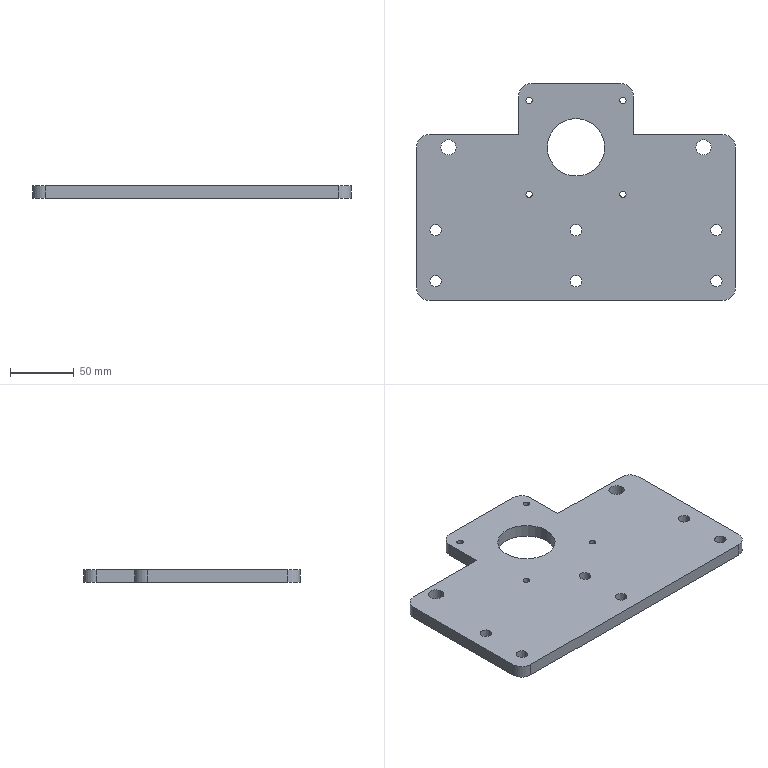Part | SolidWorks | features HoleWzd 3, LPattern 3, ICE 2, Extrusion 1, Fillet 1, MirrorPattern 1 | 1 solid | 42 faces | box 250 x 170 x 10 mm | volume 336944 mm3 | cylinder 32 | plane 10 | commonest cylinder face diameters 9 x12 5 x8 20 x6 12 x4 45 x2
STEP:
#1=CARTESIAN_POINT('',(34.27,71.77,-5.));
#2=VERTEX_POINT('',#1);
#3=CARTESIAN_POINT('',(39.27,71.77,-5.));
#4=VERTEX_POINT('',#3);
#5=CARTESIAN_POINT('',(36.77,71.77,-5.));
#6=DIRECTION('',(0.,0.,1.));
#7=DIRECTION('',(1.,0.,0.));
#8=AXIS2_PLACEMENT_3D('',#5,#6,#7);
#9=CIRCLE('',#8,2.5);
#10=EDGE_CURVE('',#2,#4,#9,.T.);
#11=ORIENTED_EDGE('',*,*,#10,.F.);
#12=CARTESIAN_POINT('',(34.27,71.77,5.));
#13=VERTEX_POINT('',#12);
#14=CARTESIAN_POINT('',(34.27,71.77,5.));
#15=DIRECTION('',(0.,0.,1.));
#16=VECTOR('',#15,1000.);
#17=LINE('',#14,#16);
#18=EDGE_CURVE('',#2,#13,#17,.T.);
#19=ORIENTED_EDGE('',*,*,#18,.T.);
#20=CARTESIAN_POINT('',(39.27,71.77,5.));
#21=VERTEX_POINT('',#20);
#22=CARTESIAN_POINT('',(36.77,71.77,5.));
#23=DIRECTION('',(0.,0.,1.));
#24=DIRECTION('',(1.,0.,0.));
#25=AXIS2_PLACEMENT_3D('',#22,#23,#24);
#26=CIRCLE('',#25,2.5);
#27=EDGE_CURVE('',#13,#21,#26,.T.);
#28=ORIENTED_EDGE('',*,*,#27,.T.);
#29=CARTESIAN_POINT('',(39.27,71.77,5.));
#30=DIRECTION('',(0.,0.,1.));
#31=VECTOR('',#30,1000.);
#32=LINE('',#29,#31);
#33=EDGE_CURVE('',#4,#21,#32,.T.);
#34=ORIENTED_EDGE('',*,*,#33,.F.);
#35=EDGE_LOOP('',(#11,#19,#28,#34));
#36=FACE_OUTER_BOUND('',#35,.T.);
#37=CARTESIAN_POINT('',(36.77,71.77,5.));
#38=DIRECTION('',(0.,0.,1.));
#39=DIRECTION('',(1.,0.,0.));
#40=AXIS2_PLACEMENT_3D('',#37,#38,#39);
#41=CYLINDRICAL_SURFACE('',#40,2.5);
#42=ADVANCED_FACE('',(#36),#41,.F.);
#43=CARTESIAN_POINT('',(34.27,-1.77,-5.));
#44=VERTEX_POINT('',#43);
#45=CARTESIAN_POINT('',(39.27,-1.77,-5.));
#46=VERTEX_POINT('',#45);
#47=CARTESIAN_POINT('',(36.77,-1.77,-5.));
#48=DIRECTION('',(0.,0.,1.));
#49=DIRECTION('',(1.,0.,0.));
#50=AXIS2_PLACEMENT_3D('',#47,#48,#49);
#51=CIRCLE('',#50,2.5);
#52=EDGE_CURVE('',#44,#46,#51,.T.);
#53=ORIENTED_EDGE('',*,*,#52,.F.);
#54=CARTESIAN_POINT('',(34.27,-1.77,5.));
#55=VERTEX_POINT('',#54);
#56=CARTESIAN_POINT('',(34.27,-1.77,5.));
#57=DIRECTION('',(0.,0.,1.));
#58=VECTOR('',#57,1000.);
#59=LINE('',#56,#58);
#60=EDGE_CURVE('',#44,#55,#59,.T.);
#61=ORIENTED_EDGE('',*,*,#60,.T.);
#62=CARTESIAN_POINT('',(39.27,-1.77,5.));
#63=VERTEX_POINT('',#62);
#64=CARTESIAN_POINT('',(36.77,-1.77,5.));
#65=DIRECTION('',(0.,0.,1.));
#66=DIRECTION('',(1.,0.,0.));
#67=AXIS2_PLACEMENT_3D('',#64,#65,#66);
#68=CIRCLE('',#67,2.5);
#69=EDGE_CURVE('',#55,#63,#68,.T.);
#70=ORIENTED_EDGE('',*,*,#69,.T.);
#71=CARTESIAN_POINT('',(39.27,-1.77,5.));
#72=DIRECTION('',(0.,0.,1.));
#73=VECTOR('',#72,1000.);
#74=LINE('',#71,#73);
#75=EDGE_CURVE('',#46,#63,#74,.T.);
#76=ORIENTED_EDGE('',*,*,#75,.F.);
#77=EDGE_LOOP('',(#53,#61,#70,#76));
#78=FACE_OUTER_BOUND('',#77,.T.);
#79=CARTESIAN_POINT('',(36.77,-1.77,5.));
#80=DIRECTION('',(0.,0.,1.));
#81=DIRECTION('',(1.,0.,0.));
#82=AXIS2_PLACEMENT_3D('',#79,#80,#81);
#83=CYLINDRICAL_SURFACE('',#82,2.5);
#84=ADVANCED_FACE('',(#78),#83,.F.);
#85=CARTESIAN_POINT('',(-39.27,-1.77,-5.));
#86=VERTEX_POINT('',#85);
#87=CARTESIAN_POINT('',(-34.27,-1.77,-5.));
#88=VERTEX_POINT('',#87);
#89=CARTESIAN_POINT('',(-36.77,-1.77,-5.));
#90=DIRECTION('',(0.,0.,1.));
#91=DIRECTION('',(1.,0.,0.));
#92=AXIS2_PLACEMENT_3D('',#89,#90,#91);
#93=CIRCLE('',#92,2.5);
#94=EDGE_CURVE('',#86,#88,#93,.T.);
#95=ORIENTED_EDGE('',*,*,#94,.F.);
#96=CARTESIAN_POINT('',(-39.27,-1.77,5.));
#97=VERTEX_POINT('',#96);
#98=CARTESIAN_POINT('',(-39.27,-1.77,5.));
#99=DIRECTION('',(0.,0.,1.));
#100=VECTOR('',#99,1000.);
#101=LINE('',#98,#100);
#102=EDGE_CURVE('',#86,#97,#101,.T.);
#103=ORIENTED_EDGE('',*,*,#102,.T.);
#104=CARTESIAN_POINT('',(-34.27,-1.77,5.));
#105=VERTEX_POINT('',#104);
#106=CARTESIAN_POINT('',(-36.77,-1.77,5.));
#107=DIRECTION('',(0.,0.,1.));
#108=DIRECTION('',(1.,0.,0.));
#109=AXIS2_PLACEMENT_3D('',#106,#107,#108);
#110=CIRCLE('',#109,2.5);
#111=EDGE_CURVE('',#97,#105,#110,.T.);
#112=ORIENTED_EDGE('',*,*,#111,.T.);
#113=CARTESIAN_POINT('',(-34.27,-1.77,5.));
#114=DIRECTION('',(0.,0.,1.));
#115=VECTOR('',#114,1000.);
#116=LINE('',#113,#115);
#117=EDGE_CURVE('',#88,#105,#116,.T.);
#118=ORIENTED_EDGE('',*,*,#117,.F.);
#119=EDGE_LOOP('',(#95,#103,#112,#118));
#120=FACE_OUTER_BOUND('',#119,.T.);
#121=CARTESIAN_POINT('',(-36.77,-1.77,5.));
#122=DIRECTION('',(0.,0.,1.));
#123=DIRECTION('',(1.,0.,0.));
#124=AXIS2_PLACEMENT_3D('',#121,#122,#123);
#125=CYLINDRICAL_SURFACE('',#124,2.5);
#126=ADVANCED_FACE('',(#120),#125,.F.);
#127=CARTESIAN_POINT('',(-39.27,71.77,-5.));
#128=VERTEX_POINT('',#127);
#129=CARTESIAN_POINT('',(-34.27,71.77,-5.));
#130=VERTEX_POINT('',#129);
#131=CARTESIAN_POINT('',(-36.77,71.77,-5.));
#132=DIRECTION('',(0.,0.,1.));
#133=DIRECTION('',(1.,0.,0.));
#134=AXIS2_PLACEMENT_3D('',#131,#132,#133);
#135=CIRCLE('',#134,2.5);
#136=EDGE_CURVE('',#128,#130,#135,.T.);
#137=ORIENTED_EDGE('',*,*,#136,.F.);
#138=CARTESIAN_POINT('',(-39.27,71.77,5.));
#139=VERTEX_POINT('',#138);
#140=CARTESIAN_POINT('',(-39.27,71.77,5.));
#141=DIRECTION('',(0.,0.,1.));
#142=VECTOR('',#141,1000.);
#143=LINE('',#140,#142);
#144=EDGE_CURVE('',#128,#139,#143,.T.);
#145=ORIENTED_EDGE('',*,*,#144,.T.);
#146=CARTESIAN_POINT('',(-34.27,71.77,5.));
#147=VERTEX_POINT('',#146);
#148=CARTESIAN_POINT('',(-36.77,71.77,5.));
#149=DIRECTION('',(0.,0.,1.));
#150=DIRECTION('',(1.,0.,0.));
#151=AXIS2_PLACEMENT_3D('',#148,#149,#150);
#152=CIRCLE('',#151,2.5);
#153=EDGE_CURVE('',#139,#147,#152,.T.);
#154=ORIENTED_EDGE('',*,*,#153,.T.);
#155=CARTESIAN_POINT('',(-34.27,71.77,5.));
#156=DIRECTION('',(0.,0.,1.));
#157=VECTOR('',#156,1000.);
#158=LINE('',#155,#157);
#159=EDGE_CURVE('',#130,#147,#158,.T.);
#160=ORIENTED_EDGE('',*,*,#159,.F.);
#161=EDGE_LOOP('',(#137,#145,#154,#160));
#162=FACE_OUTER_BOUND('',#161,.T.);
#163=CARTESIAN_POINT('',(-36.77,71.77,5.));
#164=DIRECTION('',(0.,0.,1.));
#165=DIRECTION('',(1.,0.,0.));
#166=AXIS2_PLACEMENT_3D('',#163,#164,#165);
#167=CYLINDRICAL_SURFACE('',#166,2.5);
#168=ADVANCED_FACE('',(#162),#167,.F.);
#169=CARTESIAN_POINT('',(-22.5,35.,-5.));
#170=VERTEX_POINT('',#169);
#171=CARTESIAN_POINT('',(22.5,35.,-5.));
#172=VERTEX_POINT('',#171);
#173=CARTESIAN_POINT('',(0.,35.,-5.));
#174=DIRECTION('',(0.,0.,1.));
#175=DIRECTION('',(1.,0.,0.));
#176=AXIS2_PLACEMENT_3D('',#173,#174,#175);
#177=CIRCLE('',#176,22.5);
#178=EDGE_CURVE('',#170,#172,#177,.T.);
#179=ORIENTED_EDGE('',*,*,#178,.F.);
#180=CARTESIAN_POINT('',(-22.5,35.,5.));
#181=VERTEX_POINT('',#180);
#182=CARTESIAN_POINT('',(-22.5,35.,-5.));
#183=DIRECTION('',(0.,0.,1.));
#184=VECTOR('',#183,1000.);
#185=LINE('',#182,#184);
#186=EDGE_CURVE('',#170,#181,#185,.T.);
#187=ORIENTED_EDGE('',*,*,#186,.T.);
#188=CARTESIAN_POINT('',(22.5,35.,5.));
#189=VERTEX_POINT('',#188);
#190=CARTESIAN_POINT('',(0.,35.,5.));
#191=DIRECTION('',(0.,0.,1.));
#192=DIRECTION('',(1.,0.,0.));
#193=AXIS2_PLACEMENT_3D('',#190,#191,#192);
#194=CIRCLE('',#193,22.5);
#195=EDGE_CURVE('',#181,#189,#194,.T.);
#196=ORIENTED_EDGE('',*,*,#195,.T.);
#197=CARTESIAN_POINT('',(22.5,35.,-5.));
#198=DIRECTION('',(0.,0.,1.));
#199=VECTOR('',#198,1000.);
#200=LINE('',#197,#199);
#201=EDGE_CURVE('',#172,#189,#200,.T.);
#202=ORIENTED_EDGE('',*,*,#201,.F.);
#203=EDGE_LOOP('',(#179,#187,#196,#202));
#204=FACE_OUTER_BOUND('',#203,.T.);
#205=CARTESIAN_POINT('',(0.,35.,-5.));
#206=DIRECTION('',(0.,0.,1.));
#207=DIRECTION('',(1.,0.,0.));
#208=AXIS2_PLACEMENT_3D('',#205,#206,#207);
#209=CYLINDRICAL_SURFACE('',#208,22.5);
#210=ADVANCED_FACE('',(#204),#209,.F.);
#211=CARTESIAN_POINT('',(-106.,35.,-5.));
#212=VERTEX_POINT('',#211);
#213=CARTESIAN_POINT('',(-94.,35.,-5.));
#214=VERTEX_POINT('',#213);
#215=CARTESIAN_POINT('',(-100.,35.,-5.));
#216=DIRECTION('',(0.,0.,1.));
#217=DIRECTION('',(1.,0.,0.));
#218=AXIS2_PLACEMENT_3D('',#215,#216,#217);
#219=CIRCLE('',#218,6.);
#220=EDGE_CURVE('',#212,#214,#219,.T.);
#221=ORIENTED_EDGE('',*,*,#220,.F.);
#222=CARTESIAN_POINT('',(-106.,35.,5.));
#223=VERTEX_POINT('',#222);
#224=CARTESIAN_POINT('',(-106.,35.,5.));
#225=DIRECTION('',(0.,0.,1.));
#226=VECTOR('',#225,1000.);
#227=LINE('',#224,#226);
#228=EDGE_CURVE('',#212,#223,#227,.T.);
#229=ORIENTED_EDGE('',*,*,#228,.T.);
#230=CARTESIAN_POINT('',(-94.,35.,5.));
#231=VERTEX_POINT('',#230);
#232=CARTESIAN_POINT('',(-100.,35.,5.));
#233=DIRECTION('',(0.,0.,1.));
#234=DIRECTION('',(1.,0.,0.));
#235=AXIS2_PLACEMENT_3D('',#232,#233,#234);
#236=CIRCLE('',#235,6.);
#237=EDGE_CURVE('',#223,#231,#236,.T.);
#238=ORIENTED_EDGE('',*,*,#237,.T.);
#239=CARTESIAN_POINT('',(-94.,35.,5.));
#240=DIRECTION('',(0.,0.,1.));
#241=VECTOR('',#240,1000.);
#242=LINE('',#239,#241);
#243=EDGE_CURVE('',#214,#231,#242,.T.);
#244=ORIENTED_EDGE('',*,*,#243,.F.);
#245=EDGE_LOOP('',(#221,#229,#238,#244));
#246=FACE_OUTER_BOUND('',#245,.T.);
#247=CARTESIAN_POINT('',(-100.,35.,5.));
#248=DIRECTION('',(0.,0.,1.));
#249=DIRECTION('',(1.,0.,0.));
#250=AXIS2_PLACEMENT_3D('',#247,#248,#249);
#251=CYLINDRICAL_SURFACE('',#250,6.);
#252=ADVANCED_FACE('',(#246),#251,.F.);
#253=CARTESIAN_POINT('',(94.,35.,-5.));
#254=VERTEX_POINT('',#253);
#255=CARTESIAN_POINT('',(106.,35.,-5.));
#256=VERTEX_POINT('',#255);
#257=CARTESIAN_POINT('',(100.,35.,-5.));
#258=DIRECTION('',(0.,0.,1.));
#259=DIRECTION('',(1.,0.,0.));
#260=AXIS2_PLACEMENT_3D('',#257,#258,#259);
#261=CIRCLE('',#260,6.);
#262=EDGE_CURVE('',#254,#256,#261,.T.);
#263=ORIENTED_EDGE('',*,*,#262,.F.);
#264=CARTESIAN_POINT('',(94.,35.,5.));
#265=VERTEX_POINT('',#264);
#266=CARTESIAN_POINT('',(94.,35.,5.));
#267=DIRECTION('',(0.,0.,1.));
#268=VECTOR('',#267,1000.);
#269=LINE('',#266,#268);
#270=EDGE_CURVE('',#254,#265,#269,.T.);
#271=ORIENTED_EDGE('',*,*,#270,.T.);
#272=CARTESIAN_POINT('',(106.,35.,5.));
#273=VERTEX_POINT('',#272);
#274=CARTESIAN_POINT('',(100.,35.,5.));
#275=DIRECTION('',(0.,0.,1.));
#276=DIRECTION('',(1.,0.,0.));
#277=AXIS2_PLACEMENT_3D('',#274,#275,#276);
#278=CIRCLE('',#277,6.);
#279=EDGE_CURVE('',#265,#273,#278,.T.);
#280=ORIENTED_EDGE('',*,*,#279,.T.);
#281=CARTESIAN_POINT('',(106.,35.,5.));
#282=DIRECTION('',(0.,0.,1.));
#283=VECTOR('',#282,1000.);
#284=LINE('',#281,#283);
#285=EDGE_CURVE('',#256,#273,#284,.T.);
#286=ORIENTED_EDGE('',*,*,#285,.F.);
#287=EDGE_LOOP('',(#263,#271,#280,#286));
#288=FACE_OUTER_BOUND('',#287,.T.);
#289=CARTESIAN_POINT('',(100.,35.,5.));
#290=DIRECTION('',(0.,0.,1.));
#291=DIRECTION('',(1.,0.,0.));
#292=AXIS2_PLACEMENT_3D('',#289,#290,#291);
#293=CYLINDRICAL_SURFACE('',#292,6.);
#294=ADVANCED_FACE('',(#288),#293,.F.);
#295=CARTESIAN_POINT('',(105.5,-30.,-5.));
#296=VERTEX_POINT('',#295);
#297=CARTESIAN_POINT('',(114.5,-30.,-5.));
#298=VERTEX_POINT('',#297);
#299=CARTESIAN_POINT('',(110.,-30.,-5.));
#300=DIRECTION('',(0.,0.,1.));
#301=DIRECTION('',(1.,0.,0.));
#302=AXIS2_PLACEMENT_3D('',#299,#300,#301);
#303=CIRCLE('',#302,4.5);
#304=EDGE_CURVE('',#296,#298,#303,.T.);
#305=ORIENTED_EDGE('',*,*,#304,.F.);
#306=CARTESIAN_POINT('',(105.5,-30.,5.));
#307=VERTEX_POINT('',#306);
#308=CARTESIAN_POINT('',(105.5,-30.,5.));
#309=DIRECTION('',(0.,0.,1.));
#310=VECTOR('',#309,1000.);
#311=LINE('',#308,#310);
#312=EDGE_CURVE('',#296,#307,#311,.T.);
#313=ORIENTED_EDGE('',*,*,#312,.T.);
#314=CARTESIAN_POINT('',(114.5,-30.,5.));
#315=VERTEX_POINT('',#314);
#316=CARTESIAN_POINT('',(110.,-30.,5.));
#317=DIRECTION('',(0.,0.,1.));
#318=DIRECTION('',(1.,0.,0.));
#319=AXIS2_PLACEMENT_3D('',#316,#317,#318);
#320=CIRCLE('',#319,4.5);
#321=EDGE_CURVE('',#307,#315,#320,.T.);
#322=ORIENTED_EDGE('',*,*,#321,.T.);
#323=CARTESIAN_POINT('',(114.5,-30.,5.));
#324=DIRECTION('',(0.,0.,1.));
#325=VECTOR('',#324,1000.);
#326=LINE('',#323,#325);
#327=EDGE_CURVE('',#298,#315,#326,.T.);
#328=ORIENTED_EDGE('',*,*,#327,.F.);
#329=EDGE_LOOP('',(#305,#313,#322,#328));
#330=FACE_OUTER_BOUND('',#329,.T.);
#331=CARTESIAN_POINT('',(110.,-30.,5.));
#332=DIRECTION('',(0.,0.,1.));
#333=DIRECTION('',(1.,0.,0.));
#334=AXIS2_PLACEMENT_3D('',#331,#332,#333);
#335=CYLINDRICAL_SURFACE('',#334,4.5);
#336=ADVANCED_FACE('',(#330),#335,.F.);
#337=CARTESIAN_POINT('',(-4.5,-30.,-5.));
#338=VERTEX_POINT('',#337);
#339=CARTESIAN_POINT('',(4.5,-30.,-5.));
#340=VERTEX_POINT('',#339);
#341=CARTESIAN_POINT('',(0.,-30.,-5.));
#342=DIRECTION('',(0.,0.,1.));
#343=DIRECTION('',(1.,0.,0.));
#344=AXIS2_PLACEMENT_3D('',#341,#342,#343);
#345=CIRCLE('',#344,4.5);
#346=EDGE_CURVE('',#338,#340,#345,.T.);
#347=ORIENTED_EDGE('',*,*,#346,.F.);
#348=CARTESIAN_POINT('',(-4.5,-30.,5.));
#349=VERTEX_POINT('',#348);
#350=CARTESIAN_POINT('',(-4.5,-30.,5.));
#351=DIRECTION('',(0.,0.,1.));
#352=VECTOR('',#351,1000.);
#353=LINE('',#350,#352);
#354=EDGE_CURVE('',#338,#349,#353,.T.);
#355=ORIENTED_EDGE('',*,*,#354,.T.);
#356=CARTESIAN_POINT('',(4.5,-30.,5.));
#357=VERTEX_POINT('',#356);
#358=CARTESIAN_POINT('',(0.,-30.,5.));
#359=DIRECTION('',(0.,0.,1.));
#360=DIRECTION('',(1.,0.,0.));
#361=AXIS2_PLACEMENT_3D('',#358,#359,#360);
#362=CIRCLE('',#361,4.5);
#363=EDGE_CURVE('',#349,#357,#362,.T.);
#364=ORIENTED_EDGE('',*,*,#363,.T.);
#365=CARTESIAN_POINT('',(4.5,-30.,5.));
#366=DIRECTION('',(0.,0.,1.));
#367=VECTOR('',#366,1000.);
#368=LINE('',#365,#367);
#369=EDGE_CURVE('',#340,#357,#368,.T.);
#370=ORIENTED_EDGE('',*,*,#369,.F.);
#371=EDGE_LOOP('',(#347,#355,#364,#370));
#372=FACE_OUTER_BOUND('',#371,.T.);
#373=CARTESIAN_POINT('',(0.,-30.,5.));
#374=DIRECTION('',(0.,0.,1.));
#375=DIRECTION('',(1.,0.,0.));
#376=AXIS2_PLACEMENT_3D('',#373,#374,#375);
#377=CYLINDRICAL_SURFACE('',#376,4.5);
#378=ADVANCED_FACE('',(#372),#377,.F.);
#379=CARTESIAN_POINT('',(105.5,-70.,-5.));
#380=VERTEX_POINT('',#379);
#381=CARTESIAN_POINT('',(114.5,-70.,-5.));
#382=VERTEX_POINT('',#381);
#383=CARTESIAN_POINT('',(110.,-70.,-5.));
#384=DIRECTION('',(0.,0.,1.));
#385=DIRECTION('',(1.,0.,0.));
#386=AXIS2_PLACEMENT_3D('',#383,#384,#385);
#387=CIRCLE('',#386,4.5);
#388=EDGE_CURVE('',#380,#382,#387,.T.);
#389=ORIENTED_EDGE('',*,*,#388,.F.);
#390=CARTESIAN_POINT('',(105.5,-70.,5.));
#391=VERTEX_POINT('',#390);
#392=CARTESIAN_POINT('',(105.5,-70.,5.));
#393=DIRECTION('',(0.,0.,1.));
#394=VECTOR('',#393,1000.);
#395=LINE('',#392,#394);
#396=EDGE_CURVE('',#380,#391,#395,.T.);
#397=ORIENTED_EDGE('',*,*,#396,.T.);
#398=CARTESIAN_POINT('',(114.5,-70.,5.));
#399=VERTEX_POINT('',#398);
#400=CARTESIAN_POINT('',(110.,-70.,5.));
#401=DIRECTION('',(0.,0.,1.));
#402=DIRECTION('',(1.,0.,0.));
#403=AXIS2_PLACEMENT_3D('',#400,#401,#402);
#404=CIRCLE('',#403,4.5);
#405=EDGE_CURVE('',#391,#399,#404,.T.);
#406=ORIENTED_EDGE('',*,*,#405,.T.);
#407=CARTESIAN_POINT('',(114.5,-70.,5.));
#408=DIRECTION('',(0.,0.,1.));
#409=VECTOR('',#408,1000.);
#410=LINE('',#407,#409);
#411=EDGE_CURVE('',#382,#399,#410,.T.);
#412=ORIENTED_EDGE('',*,*,#411,.F.);
#413=EDGE_LOOP('',(#389,#397,#406,#412));
#414=FACE_OUTER_BOUND('',#413,.T.);
#415=CARTESIAN_POINT('',(110.,-70.,5.));
#416=DIRECTION('',(0.,0.,1.));
#417=DIRECTION('',(1.,0.,0.));
#418=AXIS2_PLACEMENT_3D('',#415,#416,#417);
#419=CYLINDRICAL_SURFACE('',#418,4.5);
#420=ADVANCED_FACE('',(#414),#419,.F.);
#421=CARTESIAN_POINT('',(-4.5,-70.,-5.));
#422=VERTEX_POINT('',#421);
#423=CARTESIAN_POINT('',(4.5,-70.,-5.));
#424=VERTEX_POINT('',#423);
#425=CARTESIAN_POINT('',(0.,-70.,-5.));
#426=DIRECTION('',(0.,0.,1.));
#427=DIRECTION('',(1.,0.,0.));
#428=AXIS2_PLACEMENT_3D('',#425,#426,#427);
#429=CIRCLE('',#428,4.5);
#430=EDGE_CURVE('',#422,#424,#429,.T.);
#431=ORIENTED_EDGE('',*,*,#430,.F.);
#432=CARTESIAN_POINT('',(-4.5,-70.,5.));
#433=VERTEX_POINT('',#432);
#434=CARTESIAN_POINT('',(-4.5,-70.,5.));
#435=DIRECTION('',(0.,0.,1.));
#436=VECTOR('',#435,1000.);
#437=LINE('',#434,#436);
#438=EDGE_CURVE('',#422,#433,#437,.T.);
#439=ORIENTED_EDGE('',*,*,#438,.T.);
#440=CARTESIAN_POINT('',(4.5,-70.,5.));
#441=VERTEX_POINT('',#440);
#442=CARTESIAN_POINT('',(0.,-70.,5.));
#443=DIRECTION('',(0.,0.,1.));
#444=DIRECTION('',(1.,0.,0.));
#445=AXIS2_PLACEMENT_3D('',#442,#443,#444);
#446=CIRCLE('',#445,4.5);
#447=EDGE_CURVE('',#433,#441,#446,.T.);
#448=ORIENTED_EDGE('',*,*,#447,.T.);
#449=CARTESIAN_POINT('',(4.5,-70.,5.));
#450=DIRECTION('',(0.,0.,1.));
#451=VECTOR('',#450,1000.);
#452=LINE('',#449,#451);
#453=EDGE_CURVE('',#424,#441,#452,.T.);
#454=ORIENTED_EDGE('',*,*,#453,.F.);
#455=EDGE_LOOP('',(#431,#439,#448,#454));
#456=FACE_OUTER_BOUND('',#455,.T.);
#457=CARTESIAN_POINT('',(0.,-70.,5.));
#458=DIRECTION('',(0.,0.,1.));
#459=DIRECTION('',(1.,0.,0.));
#460=AXIS2_PLACEMENT_3D('',#457,#458,#459);
#461=CYLINDRICAL_SURFACE('',#460,4.5);
#462=ADVANCED_FACE('',(#456),#461,.F.);
#463=CARTESIAN_POINT('',(-114.5,-70.,-5.));
#464=VERTEX_POINT('',#463);
#465=CARTESIAN_POINT('',(-105.5,-70.,-5.));
#466=VERTEX_POINT('',#465);
#467=CARTESIAN_POINT('',(-110.,-70.,-5.));
#468=DIRECTION('',(0.,0.,1.));
#469=DIRECTION('',(1.,0.,0.));
#470=AXIS2_PLACEMENT_3D('',#467,#468,#469);
#471=CIRCLE('',#470,4.5);
#472=EDGE_CURVE('',#464,#466,#471,.T.);
#473=ORIENTED_EDGE('',*,*,#472,.F.);
#474=CARTESIAN_POINT('',(-114.5,-70.,5.));
#475=VERTEX_POINT('',#474);
#476=CARTESIAN_POINT('',(-114.5,-70.,5.));
#477=DIRECTION('',(0.,0.,1.));
#478=VECTOR('',#477,1000.);
#479=LINE('',#476,#478);
#480=EDGE_CURVE('',#464,#475,#479,.T.);
#481=ORIENTED_EDGE('',*,*,#480,.T.);
#482=CARTESIAN_POINT('',(-105.5,-70.,5.));
#483=VERTEX_POINT('',#482);
#484=CARTESIAN_POINT('',(-110.,-70.,5.));
#485=DIRECTION('',(0.,0.,1.));
#486=DIRECTION('',(1.,0.,0.));
#487=AXIS2_PLACEMENT_3D('',#484,#485,#486);
#488=CIRCLE('',#487,4.5);
#489=EDGE_CURVE('',#475,#483,#488,.T.);
#490=ORIENTED_EDGE('',*,*,#489,.T.);
#491=CARTESIAN_POINT('',(-105.5,-70.,5.));
#492=DIRECTION('',(0.,0.,1.));
#493=VECTOR('',#492,1000.);
#494=LINE('',#491,#493);
#495=EDGE_CURVE('',#466,#483,#494,.T.);
#496=ORIENTED_EDGE('',*,*,#495,.F.);
#497=EDGE_LOOP('',(#473,#481,#490,#496));
#498=FACE_OUTER_BOUND('',#497,.T.);
#499=CARTESIAN_POINT('',(-110.,-70.,5.));
#500=DIRECTION('',(0.,0.,1.));
#501=DIRECTION('',(1.,0.,0.));
#502=AXIS2_PLACEMENT_3D('',#499,#500,#501);
#503=CYLINDRICAL_SURFACE('',#502,4.5);
#504=ADVANCED_FACE('',(#498),#503,.F.);
#505=CARTESIAN_POINT('',(-114.5,-30.,-5.));
#506=VERTEX_POINT('',#505);
#507=CARTESIAN_POINT('',(-105.5,-30.,-5.));
#508=VERTEX_POINT('',#507);
#509=CARTESIAN_POINT('',(-110.,-30.,-5.));
#510=DIRECTION('',(0.,0.,1.));
#511=DIRECTION('',(1.,0.,0.));
#512=AXIS2_PLACEMENT_3D('',#509,#510,#511);
#513=CIRCLE('',#512,4.5);
#514=EDGE_CURVE('',#506,#508,#513,.T.);
#515=ORIENTED_EDGE('',*,*,#514,.F.);
#516=CARTESIAN_POINT('',(-114.5,-30.,5.));
#517=VERTEX_POINT('',#516);
#518=CARTESIAN_POINT('',(-114.5,-30.,5.));
#519=DIRECTION('',(0.,0.,1.));
#520=VECTOR('',#519,1000.);
#521=LINE('',#518,#520);
#522=EDGE_CURVE('',#506,#517,#521,.T.);
#523=ORIENTED_EDGE('',*,*,#522,.T.);
#524=CARTESIAN_POINT('',(-105.5,-30.,5.));
#525=VERTEX_POINT('',#524);
#526=CARTESIAN_POINT('',(-110.,-30.,5.));
#527=DIRECTION('',(0.,0.,1.));
#528=DIRECTION('',(1.,0.,0.));
#529=AXIS2_PLACEMENT_3D('',#526,#527,#528);
#530=CIRCLE('',#529,4.5);
#531=EDGE_CURVE('',#517,#525,#530,.T.);
#532=ORIENTED_EDGE('',*,*,#531,.T.);
#533=CARTESIAN_POINT('',(-105.5,-30.,5.));
#534=DIRECTION('',(0.,0.,1.));
#535=VECTOR('',#534,1000.);
#536=LINE('',#533,#535);
#537=EDGE_CURVE('',#508,#525,#536,.T.);
#538=ORIENTED_EDGE('',*,*,#537,.F.);
#539=EDGE_LOOP('',(#515,#523,#532,#538));
#540=FACE_OUTER_BOUND('',#539,.T.);
#541=CARTESIAN_POINT('',(-110.,-30.,5.));
#542=DIRECTION('',(0.,0.,1.));
#543=DIRECTION('',(1.,0.,0.));
#544=AXIS2_PLACEMENT_3D('',#541,#542,#543);
#545=CYLINDRICAL_SURFACE('',#544,4.5);
#546=ADVANCED_FACE('',(#540),#545,.F.);
#547=CARTESIAN_POINT('',(35.,85.,-5.));
#548=VERTEX_POINT('',#547);
#549=CARTESIAN_POINT('',(-35.,85.,-5.));
#550=VERTEX_POINT('',#549);
#551=CARTESIAN_POINT('',(-125.,85.,-5.));
#552=DIRECTION('',(-1.,0.,0.));
#553=VECTOR('',#552,1000.);
#554=LINE('',#551,#553);
#555=EDGE_CURVE('',#548,#550,#554,.T.);
#556=ORIENTED_EDGE('',*,*,#555,.T.);
#557=CARTESIAN_POINT('',(-35.,85.,5.));
#558=VERTEX_POINT('',#557);
#559=CARTESIAN_POINT('',(-35.,85.,5.));
#560=DIRECTION('',(0.,0.,1.));
#561=VECTOR('',#560,1000.);
#562=LINE('',#559,#561);
#563=EDGE_CURVE('',#550,#558,#562,.T.);
#564=ORIENTED_EDGE('',*,*,#563,.T.);
#565=CARTESIAN_POINT('',(35.,85.,5.));
#566=VERTEX_POINT('',#565);
#567=CARTESIAN_POINT('',(-125.,85.,5.));
#568=DIRECTION('',(-1.,0.,0.));
#569=VECTOR('',#568,1000.);
#570=LINE('',#567,#569);
#571=EDGE_CURVE('',#566,#558,#570,.T.);
#572=ORIENTED_EDGE('',*,*,#571,.F.);
#573=CARTESIAN_POINT('',(35.,85.,5.));
#574=DIRECTION('',(0.,0.,-1.));
#575=VECTOR('',#574,1000.);
#576=LINE('',#573,#575);
#577=EDGE_CURVE('',#566,#548,#576,.T.);
#578=ORIENTED_EDGE('',*,*,#577,.T.);
#579=EDGE_LOOP('',(#556,#564,#572,#578));
#580=FACE_OUTER_BOUND('',#579,.T.);
#581=CARTESIAN_POINT('',(-125.,85.,5.));
#582=DIRECTION('',(0.,-1.,0.));
#583=DIRECTION('',(0.,0.,-1.));
#584=AXIS2_PLACEMENT_3D('',#581,#582,#583);
#585=PLANE('',#584);
#586=ADVANCED_FACE('',(#580),#585,.F.);
#587=CARTESIAN_POINT('',(-125.,35.,-5.));
#588=VERTEX_POINT('',#587);
#589=CARTESIAN_POINT('',(-125.,-75.,-5.));
#590=VERTEX_POINT('',#589);
#591=CARTESIAN_POINT('',(-125.,85.,-5.));
#592=DIRECTION('',(0.,-1.,0.));
#593=VECTOR('',#592,1000.);
#594=LINE('',#591,#593);
#595=EDGE_CURVE('',#588,#590,#594,.T.);
#596=ORIENTED_EDGE('',*,*,#595,.T.);
#597=CARTESIAN_POINT('',(-125.,-75.,5.));
#598=VERTEX_POINT('',#597);
#599=CARTESIAN_POINT('',(-125.,-75.,5.));
#600=DIRECTION('',(0.,0.,1.));
#601=VECTOR('',#600,1000.);
#602=LINE('',#599,#601);
#603=EDGE_CURVE('',#590,#598,#602,.T.);
#604=ORIENTED_EDGE('',*,*,#603,.T.);
#605=CARTESIAN_POINT('',(-125.,35.,5.));
#606=VERTEX_POINT('',#605);
#607=CARTESIAN_POINT('',(-125.,85.,5.));
#608=DIRECTION('',(0.,-1.,0.));
#609=VECTOR('',#608,1000.);
#610=LINE('',#607,#609);
#611=EDGE_CURVE('',#606,#598,#610,.T.);
#612=ORIENTED_EDGE('',*,*,#611,.F.);
#613=CARTESIAN_POINT('',(-125.,35.,-5.));
#614=DIRECTION('',(0.,0.,-1.));
#615=VECTOR('',#614,1000.);
#616=LINE('',#613,#615);
#617=EDGE_CURVE('',#606,#588,#616,.T.);
#618=ORIENTED_EDGE('',*,*,#617,.T.);
#619=EDGE_LOOP('',(#596,#604,#612,#618));
#620=FACE_OUTER_BOUND('',#619,.T.);
#621=CARTESIAN_POINT('',(-125.,85.,5.));
#622=DIRECTION('',(1.,0.,0.));
#623=DIRECTION('',(0.,0.,-1.));
#624=AXIS2_PLACEMENT_3D('',#621,#622,#623);
#625=PLANE('',#624);
#626=ADVANCED_FACE('',(#620),#625,.F.);
#627=CARTESIAN_POINT('',(36.77,71.77,5.));
#628=DIRECTION('',(0.,0.,1.));
#629=DIRECTION('',(1.,0.,0.));
#630=AXIS2_PLACEMENT_3D('',#627,#628,#629);
#631=CIRCLE('',#630,2.5);
#632=EDGE_CURVE('',#21,#13,#631,.T.);
#633=ORIENTED_EDGE('',*,*,#632,.F.);
#634=ORIENTED_EDGE('',*,*,#27,.F.);
#635=EDGE_LOOP('',(#633,#634));
#636=FACE_BOUND('',#635,.T.);
#637=CARTESIAN_POINT('',(36.77,-1.77,5.));
#638=DIRECTION('',(0.,0.,1.));
#639=DIRECTION('',(1.,0.,0.));
#640=AXIS2_PLACEMENT_3D('',#637,#638,#639);
#641=CIRCLE('',#640,2.5);
#642=EDGE_CURVE('',#63,#55,#641,.T.);
#643=ORIENTED_EDGE('',*,*,#642,.F.);
#644=ORIENTED_EDGE('',*,*,#69,.F.);
#645=EDGE_LOOP('',(#643,#644));
#646=FACE_BOUND('',#645,.T.);
#647=CARTESIAN_POINT('',(-36.77,-1.77,5.));
#648=DIRECTION('',(0.,0.,1.));
#649=DIRECTION('',(1.,0.,0.));
#650=AXIS2_PLACEMENT_3D('',#647,#648,#649);
#651=CIRCLE('',#650,2.5);
#652=EDGE_CURVE('',#105,#97,#651,.T.);
#653=ORIENTED_EDGE('',*,*,#652,.F.);
#654=ORIENTED_EDGE('',*,*,#111,.F.);
#655=EDGE_LOOP('',(#653,#654));
#656=FACE_BOUND('',#655,.T.);
#657=CARTESIAN_POINT('',(-36.77,71.77,5.));
#658=DIRECTION('',(0.,0.,1.));
#659=DIRECTION('',(1.,0.,0.));
#660=AXIS2_PLACEMENT_3D('',#657,#658,#659);
#661=CIRCLE('',#660,2.5);
#662=EDGE_CURVE('',#147,#139,#661,.T.);
#663=ORIENTED_EDGE('',*,*,#662,.F.);
#664=ORIENTED_EDGE('',*,*,#153,.F.);
#665=EDGE_LOOP('',(#663,#664));
#666=FACE_BOUND('',#665,.T.);
#667=CARTESIAN_POINT('',(0.,35.,5.));
#668=DIRECTION('',(0.,0.,1.));
#669=DIRECTION('',(1.,0.,0.));
#670=AXIS2_PLACEMENT_3D('',#667,#668,#669);
#671=CIRCLE('',#670,22.5);
#672=EDGE_CURVE('',#189,#181,#671,.T.);
#673=ORIENTED_EDGE('',*,*,#672,.F.);
#674=ORIENTED_EDGE('',*,*,#195,.F.);
#675=EDGE_LOOP('',(#673,#674));
#676=FACE_BOUND('',#675,.T.);
#677=CARTESIAN_POINT('',(-100.,35.,5.));
#678=DIRECTION('',(0.,0.,1.));
#679=DIRECTION('',(1.,0.,0.));
#680=AXIS2_PLACEMENT_3D('',#677,#678,#679);
#681=CIRCLE('',#680,6.);
#682=EDGE_CURVE('',#231,#223,#681,.T.);
#683=ORIENTED_EDGE('',*,*,#682,.F.);
#684=ORIENTED_EDGE('',*,*,#237,.F.);
#685=EDGE_LOOP('',(#683,#684));
#686=FACE_BOUND('',#685,.T.);
#687=CARTESIAN_POINT('',(100.,35.,5.));
#688=DIRECTION('',(0.,0.,1.));
#689=DIRECTION('',(1.,0.,0.));
#690=AXIS2_PLACEMENT_3D('',#687,#688,#689);
#691=CIRCLE('',#690,6.);
#692=EDGE_CURVE('',#273,#265,#691,.T.);
#693=ORIENTED_EDGE('',*,*,#692,.F.);
#694=ORIENTED_EDGE('',*,*,#279,.F.);
#695=EDGE_LOOP('',(#693,#694));
#696=FACE_BOUND('',#695,.T.);
#697=CARTESIAN_POINT('',(0.,-30.,5.));
#698=DIRECTION('',(0.,0.,1.));
#699=DIRECTION('',(1.,0.,0.));
#700=AXIS2_PLACEMENT_3D('',#697,#698,#699);
#701=CIRCLE('',#700,4.5);
#702=EDGE_CURVE('',#357,#349,#701,.T.);
#703=ORIENTED_EDGE('',*,*,#702,.F.);
#704=ORIENTED_EDGE('',*,*,#363,.F.);
#705=EDGE_LOOP('',(#703,#704));
#706=FACE_BOUND('',#705,.T.);
#707=CARTESIAN_POINT('',(0.,-70.,5.));
#708=DIRECTION('',(0.,0.,1.));
#709=DIRECTION('',(1.,0.,0.));
#710=AXIS2_PLACEMENT_3D('',#707,#708,#709);
#711=CIRCLE('',#710,4.5);
#712=EDGE_CURVE('',#441,#433,#711,.T.);
#713=ORIENTED_EDGE('',*,*,#712,.F.);
#714=ORIENTED_EDGE('',*,*,#447,.F.);
#715=EDGE_LOOP('',(#713,#714));
#716=FACE_BOUND('',#715,.T.);
#717=CARTESIAN_POINT('',(-110.,-70.,5.));
#718=DIRECTION('',(0.,0.,1.));
#719=DIRECTION('',(1.,0.,0.));
#720=AXIS2_PLACEMENT_3D('',#717,#718,#719);
#721=CIRCLE('',#720,4.5);
#722=EDGE_CURVE('',#483,#475,#721,.T.);
#723=ORIENTED_EDGE('',*,*,#722,.F.);
#724=ORIENTED_EDGE('',*,*,#489,.F.);
#725=EDGE_LOOP('',(#723,#724));
#726=FACE_BOUND('',#725,.T.);
#727=CARTESIAN_POINT('',(-110.,-30.,5.));
#728=DIRECTION('',(0.,0.,1.));
#729=DIRECTION('',(1.,0.,0.));
#730=AXIS2_PLACEMENT_3D('',#727,#728,#729);
#731=CIRCLE('',#730,4.5);
#732=EDGE_CURVE('',#525,#517,#731,.T.);
#733=ORIENTED_EDGE('',*,*,#732,.F.);
#734=ORIENTED_EDGE('',*,*,#531,.F.);
#735=EDGE_LOOP('',(#733,#734));
#736=FACE_BOUND('',#735,.T.);
#737=ORIENTED_EDGE('',*,*,#611,.T.);
#738=CARTESIAN_POINT('',(-115.,-85.,5.));
#739=VERTEX_POINT('',#738);
#740=CARTESIAN_POINT('',(-115.,-75.,5.));
#741=DIRECTION('',(0.,0.,1.));
#742=DIRECTION('',(1.,0.,0.));
#743=AXIS2_PLACEMENT_3D('',#740,#741,#742);
#744=CIRCLE('',#743,10.);
#745=EDGE_CURVE('',#598,#739,#744,.T.);
#746=ORIENTED_EDGE('',*,*,#745,.T.);
#747=CARTESIAN_POINT('',(115.,-85.,5.));
#748=VERTEX_POINT('',#747);
#749=CARTESIAN_POINT('',(-125.,-85.,5.));
#750=DIRECTION('',(1.,0.,0.));
#751=VECTOR('',#750,1000.);
#752=LINE('',#749,#751);
#753=EDGE_CURVE('',#739,#748,#752,.T.);
#754=ORIENTED_EDGE('',*,*,#753,.T.);
#755=CARTESIAN_POINT('',(125.,-75.,5.));
#756=VERTEX_POINT('',#755);
#757=CARTESIAN_POINT('',(115.,-75.,5.));
#758=DIRECTION('',(0.,0.,1.));
#759=DIRECTION('',(1.,0.,0.));
#760=AXIS2_PLACEMENT_3D('',#757,#758,#759);
#761=CIRCLE('',#760,10.);
#762=EDGE_CURVE('',#748,#756,#761,.T.);
#763=ORIENTED_EDGE('',*,*,#762,.T.);
#764=CARTESIAN_POINT('',(125.,35.,5.));
#765=VERTEX_POINT('',#764);
#766=CARTESIAN_POINT('',(125.,85.,5.));
#767=DIRECTION('',(0.,1.,0.));
#768=VECTOR('',#767,1000.);
#769=LINE('',#766,#768);
#770=EDGE_CURVE('',#756,#765,#769,.T.);
#771=ORIENTED_EDGE('',*,*,#770,.T.);
#772=CARTESIAN_POINT('',(115.,45.,5.));
#773=VERTEX_POINT('',#772);
#774=CARTESIAN_POINT('',(115.,35.,5.));
#775=DIRECTION('',(0.,0.,1.));
#776=DIRECTION('',(1.,0.,0.));
#777=AXIS2_PLACEMENT_3D('',#774,#775,#776);
#778=CIRCLE('',#777,10.);
#779=EDGE_CURVE('',#765,#773,#778,.T.);
#780=ORIENTED_EDGE('',*,*,#779,.T.);
#781=CARTESIAN_POINT('',(45.,45.,5.));
#782=VERTEX_POINT('',#781);
#783=CARTESIAN_POINT('',(125.,45.,5.));
#784=DIRECTION('',(1.,0.,0.));
#785=VECTOR('',#784,1000.);
#786=LINE('',#783,#785);
#787=EDGE_CURVE('',#782,#773,#786,.T.);
#788=ORIENTED_EDGE('',*,*,#787,.F.);
#789=CARTESIAN_POINT('',(45.,75.,5.));
#790=VERTEX_POINT('',#789);
#791=CARTESIAN_POINT('',(45.,85.,5.));
#792=DIRECTION('',(0.,-1.,0.));
#793=VECTOR('',#792,1000.);
#794=LINE('',#791,#793);
#795=EDGE_CURVE('',#790,#782,#794,.T.);
#796=ORIENTED_EDGE('',*,*,#795,.F.);
#797=CARTESIAN_POINT('',(35.,75.,5.));
#798=DIRECTION('',(0.,0.,1.));
#799=DIRECTION('',(1.,0.,0.));
#800=AXIS2_PLACEMENT_3D('',#797,#798,#799);
#801=CIRCLE('',#800,10.);
#802=EDGE_CURVE('',#790,#566,#801,.T.);
#803=ORIENTED_EDGE('',*,*,#802,.T.);
#804=ORIENTED_EDGE('',*,*,#571,.T.);
#805=CARTESIAN_POINT('',(-45.,75.,5.));
#806=VERTEX_POINT('',#805);
#807=CARTESIAN_POINT('',(-35.,75.,5.));
#808=DIRECTION('',(0.,0.,1.));
#809=DIRECTION('',(1.,0.,0.));
#810=AXIS2_PLACEMENT_3D('',#807,#808,#809);
#811=CIRCLE('',#810,10.);
#812=EDGE_CURVE('',#558,#806,#811,.T.);
#813=ORIENTED_EDGE('',*,*,#812,.T.);
#814=CARTESIAN_POINT('',(-45.,45.,5.));
#815=VERTEX_POINT('',#814);
#816=CARTESIAN_POINT('',(-45.,85.,5.));
#817=DIRECTION('',(0.,-1.,0.));
#818=VECTOR('',#817,1000.);
#819=LINE('',#816,#818);
#820=EDGE_CURVE('',#806,#815,#819,.T.);
#821=ORIENTED_EDGE('',*,*,#820,.T.);
#822=CARTESIAN_POINT('',(-115.,45.,5.));
#823=VERTEX_POINT('',#822);
#824=CARTESIAN_POINT('',(-125.,45.,5.));
#825=DIRECTION('',(-1.,0.,0.));
#826=VECTOR('',#825,1000.);
#827=LINE('',#824,#826);
#828=EDGE_CURVE('',#815,#823,#827,.T.);
#829=ORIENTED_EDGE('',*,*,#828,.T.);
#830=CARTESIAN_POINT('',(-115.,35.,5.));
#831=DIRECTION('',(0.,0.,1.));
#832=DIRECTION('',(1.,0.,0.));
#833=AXIS2_PLACEMENT_3D('',#830,#831,#832);
#834=CIRCLE('',#833,10.);
#835=EDGE_CURVE('',#823,#606,#834,.T.);
#836=ORIENTED_EDGE('',*,*,#835,.T.);
#837=EDGE_LOOP('',(#737,#746,#754,#763,#771,#780,#788,#796,#803,#804,#813,#821,#829,#836));
#838=FACE_OUTER_BOUND('',#837,.T.);
#839=CARTESIAN_POINT('',(110.,-70.,5.));
#840=DIRECTION('',(0.,0.,1.));
#841=DIRECTION('',(1.,0.,0.));
#842=AXIS2_PLACEMENT_3D('',#839,#840,#841);
#843=CIRCLE('',#842,4.5);
#844=EDGE_CURVE('',#399,#391,#843,.T.);
#845=ORIENTED_EDGE('',*,*,#844,.F.);
#846=ORIENTED_EDGE('',*,*,#405,.F.);
#847=EDGE_LOOP('',(#845,#846));
#848=FACE_BOUND('',#847,.T.);
#849=CARTESIAN_POINT('',(110.,-30.,5.));
#850=DIRECTION('',(0.,0.,1.));
#851=DIRECTION('',(1.,0.,0.));
#852=AXIS2_PLACEMENT_3D('',#849,#850,#851);
#853=CIRCLE('',#852,4.5);
#854=EDGE_CURVE('',#315,#307,#853,.T.);
#855=ORIENTED_EDGE('',*,*,#854,.F.);
#856=ORIENTED_EDGE('',*,*,#321,.F.);
#857=EDGE_LOOP('',(#855,#856));
#858=FACE_BOUND('',#857,.T.);
#859=CARTESIAN_POINT('',(0.,0.,5.));
#860=DIRECTION('',(0.,0.,1.));
#861=DIRECTION('',(1.,0.,0.));
#862=AXIS2_PLACEMENT_3D('',#859,#860,#861);
#863=PLANE('',#862);
#864=ADVANCED_FACE('',(#636,#646,#656,#666,#676,#686,#696,#706,#716,#726,#736,#838,#848,#858),#863,.T.);
#865=CARTESIAN_POINT('',(36.77,71.77,-5.));
#866=DIRECTION('',(0.,0.,1.));
#867=DIRECTION('',(1.,0.,0.));
#868=AXIS2_PLACEMENT_3D('',#865,#866,#867);
#869=CIRCLE('',#868,2.5);
#870=EDGE_CURVE('',#4,#2,#869,.T.);
#871=ORIENTED_EDGE('',*,*,#870,.T.);
#872=ORIENTED_EDGE('',*,*,#10,.T.);
#873=EDGE_LOOP('',(#871,#872));
#874=FACE_BOUND('',#873,.T.);
#875=CARTESIAN_POINT('',(36.77,-1.77,-5.));
#876=DIRECTION('',(0.,0.,1.));
#877=DIRECTION('',(1.,0.,0.));
#878=AXIS2_PLACEMENT_3D('',#875,#876,#877);
#879=CIRCLE('',#878,2.5);
#880=EDGE_CURVE('',#46,#44,#879,.T.);
#881=ORIENTED_EDGE('',*,*,#880,.T.);
#882=ORIENTED_EDGE('',*,*,#52,.T.);
#883=EDGE_LOOP('',(#881,#882));
#884=FACE_BOUND('',#883,.T.);
#885=CARTESIAN_POINT('',(-36.77,-1.77,-5.));
#886=DIRECTION('',(0.,0.,1.));
#887=DIRECTION('',(1.,0.,0.));
#888=AXIS2_PLACEMENT_3D('',#885,#886,#887);
#889=CIRCLE('',#888,2.5);
#890=EDGE_CURVE('',#88,#86,#889,.T.);
#891=ORIENTED_EDGE('',*,*,#890,.T.);
#892=ORIENTED_EDGE('',*,*,#94,.T.);
#893=EDGE_LOOP('',(#891,#892));
#894=FACE_BOUND('',#893,.T.);
#895=CARTESIAN_POINT('',(-36.77,71.77,-5.));
#896=DIRECTION('',(0.,0.,1.));
#897=DIRECTION('',(1.,0.,0.));
#898=AXIS2_PLACEMENT_3D('',#895,#896,#897);
#899=CIRCLE('',#898,2.5);
#900=EDGE_CURVE('',#130,#128,#899,.T.);
#901=ORIENTED_EDGE('',*,*,#900,.T.);
#902=ORIENTED_EDGE('',*,*,#136,.T.);
#903=EDGE_LOOP('',(#901,#902));
#904=FACE_BOUND('',#903,.T.);
#905=CARTESIAN_POINT('',(0.,35.,-5.));
#906=DIRECTION('',(0.,0.,1.));
#907=DIRECTION('',(1.,0.,0.));
#908=AXIS2_PLACEMENT_3D('',#905,#906,#907);
#909=CIRCLE('',#908,22.5);
#910=EDGE_CURVE('',#172,#170,#909,.T.);
#911=ORIENTED_EDGE('',*,*,#910,.T.);
#912=ORIENTED_EDGE('',*,*,#178,.T.);
#913=EDGE_LOOP('',(#911,#912));
#914=FACE_BOUND('',#913,.T.);
#915=CARTESIAN_POINT('',(-100.,35.,-5.));
#916=DIRECTION('',(0.,0.,1.));
#917=DIRECTION('',(1.,0.,0.));
#918=AXIS2_PLACEMENT_3D('',#915,#916,#917);
#919=CIRCLE('',#918,6.);
#920=EDGE_CURVE('',#214,#212,#919,.T.);
#921=ORIENTED_EDGE('',*,*,#920,.T.);
#922=ORIENTED_EDGE('',*,*,#220,.T.);
#923=EDGE_LOOP('',(#921,#922));
#924=FACE_BOUND('',#923,.T.);
#925=CARTESIAN_POINT('',(100.,35.,-5.));
#926=DIRECTION('',(0.,0.,1.));
#927=DIRECTION('',(1.,0.,0.));
#928=AXIS2_PLACEMENT_3D('',#925,#926,#927);
#929=CIRCLE('',#928,6.);
#930=EDGE_CURVE('',#256,#254,#929,.T.);
#931=ORIENTED_EDGE('',*,*,#930,.T.);
#932=ORIENTED_EDGE('',*,*,#262,.T.);
#933=EDGE_LOOP('',(#931,#932));
#934=FACE_BOUND('',#933,.T.);
#935=CARTESIAN_POINT('',(0.,-30.,-5.));
#936=DIRECTION('',(0.,0.,1.));
#937=DIRECTION('',(1.,0.,0.));
#938=AXIS2_PLACEMENT_3D('',#935,#936,#937);
#939=CIRCLE('',#938,4.5);
#940=EDGE_CURVE('',#340,#338,#939,.T.);
#941=ORIENTED_EDGE('',*,*,#940,.T.);
#942=ORIENTED_EDGE('',*,*,#346,.T.);
#943=EDGE_LOOP('',(#941,#942));
#944=FACE_BOUND('',#943,.T.);
#945=CARTESIAN_POINT('',(0.,-70.,-5.));
#946=DIRECTION('',(0.,0.,1.));
#947=DIRECTION('',(1.,0.,0.));
#948=AXIS2_PLACEMENT_3D('',#945,#946,#947);
#949=CIRCLE('',#948,4.5);
#950=EDGE_CURVE('',#424,#422,#949,.T.);
#951=ORIENTED_EDGE('',*,*,#950,.T.);
#952=ORIENTED_EDGE('',*,*,#430,.T.);
#953=EDGE_LOOP('',(#951,#952));
#954=FACE_BOUND('',#953,.T.);
#955=CARTESIAN_POINT('',(-110.,-70.,-5.));
#956=DIRECTION('',(0.,0.,1.));
#957=DIRECTION('',(1.,0.,0.));
#958=AXIS2_PLACEMENT_3D('',#955,#956,#957);
#959=CIRCLE('',#958,4.5);
#960=EDGE_CURVE('',#466,#464,#959,.T.);
#961=ORIENTED_EDGE('',*,*,#960,.T.);
#962=ORIENTED_EDGE('',*,*,#472,.T.);
#963=EDGE_LOOP('',(#961,#962));
#964=FACE_BOUND('',#963,.T.);
#965=CARTESIAN_POINT('',(-110.,-30.,-5.));
#966=DIRECTION('',(0.,0.,1.));
#967=DIRECTION('',(1.,0.,0.));
#968=AXIS2_PLACEMENT_3D('',#965,#966,#967);
#969=CIRCLE('',#968,4.5);
#970=EDGE_CURVE('',#508,#506,#969,.T.);
#971=ORIENTED_EDGE('',*,*,#970,.T.);
#972=ORIENTED_EDGE('',*,*,#514,.T.);
#973=EDGE_LOOP('',(#971,#972));
#974=FACE_BOUND('',#973,.T.);
#975=CARTESIAN_POINT('',(-115.,-85.,-5.));
#976=VERTEX_POINT('',#975);
#977=CARTESIAN_POINT('',(115.,-85.,-5.));
#978=VERTEX_POINT('',#977);
#979=CARTESIAN_POINT('',(-125.,-85.,-5.));
#980=DIRECTION('',(1.,0.,0.));
#981=VECTOR('',#980,1000.);
#982=LINE('',#979,#981);
#983=EDGE_CURVE('',#976,#978,#982,.T.);
#984=ORIENTED_EDGE('',*,*,#983,.F.);
#985=CARTESIAN_POINT('',(-115.,-75.,-5.));
#986=DIRECTION('',(0.,0.,-1.));
#987=DIRECTION('',(1.,0.,0.));
#988=AXIS2_PLACEMENT_3D('',#985,#986,#987);
#989=CIRCLE('',#988,10.);
#990=EDGE_CURVE('',#976,#590,#989,.T.);
#991=ORIENTED_EDGE('',*,*,#990,.T.);
#992=ORIENTED_EDGE('',*,*,#595,.F.);
#993=CARTESIAN_POINT('',(-115.,45.,-5.));
#994=VERTEX_POINT('',#993);
#995=CARTESIAN_POINT('',(-115.,35.,-5.));
#996=DIRECTION('',(0.,0.,-1.));
#997=DIRECTION('',(1.,0.,0.));
#998=AXIS2_PLACEMENT_3D('',#995,#996,#997);
#999=CIRCLE('',#998,10.);
#1000=EDGE_CURVE('',#588,#994,#999,.T.);
#1001=ORIENTED_EDGE('',*,*,#1000,.T.);
#1002=CARTESIAN_POINT('',(-45.,45.,-5.));
#1003=VERTEX_POINT('',#1002);
#1004=CARTESIAN_POINT('',(-125.,45.,-5.));
#1005=DIRECTION('',(-1.,0.,0.));
#1006=VECTOR('',#1005,1000.);
#1007=LINE('',#1004,#1006);
#1008=EDGE_CURVE('',#1003,#994,#1007,.T.);
#1009=ORIENTED_EDGE('',*,*,#1008,.F.);
#1010=CARTESIAN_POINT('',(-45.,75.,-5.));
#1011=VERTEX_POINT('',#1010);
#1012=CARTESIAN_POINT('',(-45.,85.,-5.));
#1013=DIRECTION('',(0.,-1.,0.));
#1014=VECTOR('',#1013,1000.);
#1015=LINE('',#1012,#1014);
#1016=EDGE_CURVE('',#1011,#1003,#1015,.T.);
#1017=ORIENTED_EDGE('',*,*,#1016,.F.);
#1018=CARTESIAN_POINT('',(-35.,75.,-5.));
#1019=DIRECTION('',(0.,0.,-1.));
#1020=DIRECTION('',(1.,0.,0.));
#1021=AXIS2_PLACEMENT_3D('',#1018,#1019,#1020);
#1022=CIRCLE('',#1021,10.);
#1023=EDGE_CURVE('',#1011,#550,#1022,.T.);
#1024=ORIENTED_EDGE('',*,*,#1023,.T.);
#1025=ORIENTED_EDGE('',*,*,#555,.F.);
#1026=CARTESIAN_POINT('',(45.,75.,-5.));
#1027=VERTEX_POINT('',#1026);
#1028=CARTESIAN_POINT('',(35.,75.,-5.));
#1029=DIRECTION('',(0.,0.,-1.));
#1030=DIRECTION('',(1.,0.,0.));
#1031=AXIS2_PLACEMENT_3D('',#1028,#1029,#1030);
#1032=CIRCLE('',#1031,10.);
#1033=EDGE_CURVE('',#548,#1027,#1032,.T.);
#1034=ORIENTED_EDGE('',*,*,#1033,.T.);
#1035=CARTESIAN_POINT('',(45.,45.,-5.));
#1036=VERTEX_POINT('',#1035);
#1037=CARTESIAN_POINT('',(45.,85.,-5.));
#1038=DIRECTION('',(0.,-1.,0.));
#1039=VECTOR('',#1038,1000.);
#1040=LINE('',#1037,#1039);
#1041=EDGE_CURVE('',#1027,#1036,#1040,.T.);
#1042=ORIENTED_EDGE('',*,*,#1041,.T.);
#1043=CARTESIAN_POINT('',(115.,45.,-5.));
#1044=VERTEX_POINT('',#1043);
#1045=CARTESIAN_POINT('',(125.,45.,-5.));
#1046=DIRECTION('',(1.,0.,0.));
#1047=VECTOR('',#1046,1000.);
#1048=LINE('',#1045,#1047);
#1049=EDGE_CURVE('',#1036,#1044,#1048,.T.);
#1050=ORIENTED_EDGE('',*,*,#1049,.T.);
#1051=CARTESIAN_POINT('',(125.,35.,-5.));
#1052=VERTEX_POINT('',#1051);
#1053=CARTESIAN_POINT('',(115.,35.,-5.));
#1054=DIRECTION('',(0.,0.,-1.));
#1055=DIRECTION('',(1.,0.,0.));
#1056=AXIS2_PLACEMENT_3D('',#1053,#1054,#1055);
#1057=CIRCLE('',#1056,10.);
#1058=EDGE_CURVE('',#1044,#1052,#1057,.T.);
#1059=ORIENTED_EDGE('',*,*,#1058,.T.);
#1060=CARTESIAN_POINT('',(125.,-75.,-5.));
#1061=VERTEX_POINT('',#1060);
#1062=CARTESIAN_POINT('',(125.,85.,-5.));
#1063=DIRECTION('',(0.,1.,0.));
#1064=VECTOR('',#1063,1000.);
#1065=LINE('',#1062,#1064);
#1066=EDGE_CURVE('',#1061,#1052,#1065,.T.);
#1067=ORIENTED_EDGE('',*,*,#1066,.F.);
#1068=CARTESIAN_POINT('',(115.,-75.,-5.));
#1069=DIRECTION('',(0.,0.,-1.));
#1070=DIRECTION('',(1.,0.,0.));
#1071=AXIS2_PLACEMENT_3D('',#1068,#1069,#1070);
#1072=CIRCLE('',#1071,10.);
#1073=EDGE_CURVE('',#1061,#978,#1072,.T.);
#1074=ORIENTED_EDGE('',*,*,#1073,.T.);
#1075=EDGE_LOOP('',(#984,#991,#992,#1001,#1009,#1017,#1024,#1025,#1034,#1042,#1050,#1059,#1067,#1074));
#1076=FACE_OUTER_BOUND('',#1075,.T.);
#1077=CARTESIAN_POINT('',(110.,-70.,-5.));
#1078=DIRECTION('',(0.,0.,1.));
#1079=DIRECTION('',(1.,0.,0.));
#1080=AXIS2_PLACEMENT_3D('',#1077,#1078,#1079);
#1081=CIRCLE('',#1080,4.5);
#1082=EDGE_CURVE('',#382,#380,#1081,.T.);
#1083=ORIENTED_EDGE('',*,*,#1082,.T.);
#1084=ORIENTED_EDGE('',*,*,#388,.T.);
#1085=EDGE_LOOP('',(#1083,#1084));
#1086=FACE_BOUND('',#1085,.T.);
#1087=CARTESIAN_POINT('',(110.,-30.,-5.));
#1088=DIRECTION('',(0.,0.,1.));
#1089=DIRECTION('',(1.,0.,0.));
#1090=AXIS2_PLACEMENT_3D('',#1087,#1088,#1089);
#1091=CIRCLE('',#1090,4.5);
#1092=EDGE_CURVE('',#298,#296,#1091,.T.);
#1093=ORIENTED_EDGE('',*,*,#1092,.T.);
#1094=ORIENTED_EDGE('',*,*,#304,.T.);
#1095=EDGE_LOOP('',(#1093,#1094));
#1096=FACE_BOUND('',#1095,.T.);
#1097=CARTESIAN_POINT('',(0.,0.,-5.));
#1098=DIRECTION('',(0.,0.,1.));
#1099=DIRECTION('',(1.,0.,0.));
#1100=AXIS2_PLACEMENT_3D('',#1097,#1098,#1099);
#1101=PLANE('',#1100);
#1102=ADVANCED_FACE('',(#874,#884,#894,#904,#914,#924,#934,#944,#954,#964,#974,#1076,#1086,#1096),#1101,.F.);
#1103=ORIENTED_EDGE('',*,*,#770,.F.);
#1104=CARTESIAN_POINT('',(125.,-75.,5.));
#1105=DIRECTION('',(0.,0.,-1.));
#1106=VECTOR('',#1105,1000.);
#1107=LINE('',#1104,#1106);
#1108=EDGE_CURVE('',#756,#1061,#1107,.T.);
#1109=ORIENTED_EDGE('',*,*,#1108,.T.);
#1110=ORIENTED_EDGE('',*,*,#1066,.T.);
#1111=CARTESIAN_POINT('',(125.,35.,5.));
#1112=DIRECTION('',(0.,0.,1.));
#1113=VECTOR('',#1112,1000.);
#1114=LINE('',#1111,#1113);
#1115=EDGE_CURVE('',#1052,#765,#1114,.T.);
#1116=ORIENTED_EDGE('',*,*,#1115,.T.);
#1117=EDGE_LOOP('',(#1103,#1109,#1110,#1116));
#1118=FACE_OUTER_BOUND('',#1117,.T.);
#1119=CARTESIAN_POINT('',(125.,85.,5.));
#1120=DIRECTION('',(-1.,0.,0.));
#1121=DIRECTION('',(0.,0.,1.));
#1122=AXIS2_PLACEMENT_3D('',#1119,#1120,#1121);
#1123=PLANE('',#1122);
#1124=ADVANCED_FACE('',(#1118),#1123,.F.);
#1125=ORIENTED_EDGE('',*,*,#753,.F.);
#1126=CARTESIAN_POINT('',(-115.,-85.,5.));
#1127=DIRECTION('',(0.,0.,-1.));
#1128=VECTOR('',#1127,1000.);
#1129=LINE('',#1126,#1128);
#1130=EDGE_CURVE('',#739,#976,#1129,.T.);
#1131=ORIENTED_EDGE('',*,*,#1130,.T.);
#1132=ORIENTED_EDGE('',*,*,#983,.T.);
#1133=CARTESIAN_POINT('',(115.,-85.,5.));
#1134=DIRECTION('',(0.,0.,1.));
#1135=VECTOR('',#1134,1000.);
#1136=LINE('',#1133,#1135);
#1137=EDGE_CURVE('',#978,#748,#1136,.T.);
#1138=ORIENTED_EDGE('',*,*,#1137,.T.);
#1139=EDGE_LOOP('',(#1125,#1131,#1132,#1138));
#1140=FACE_OUTER_BOUND('',#1139,.T.);
#1141=CARTESIAN_POINT('',(-125.,-85.,5.));
#1142=DIRECTION('',(0.,1.,0.));
#1143=DIRECTION('',(0.,0.,1.));
#1144=AXIS2_PLACEMENT_3D('',#1141,#1142,#1143);
#1145=PLANE('',#1144);
#1146=ADVANCED_FACE('',(#1140),#1145,.F.);
#1147=ORIENTED_EDGE('',*,*,#787,.T.);
#1148=CARTESIAN_POINT('',(115.,45.,-5.));
#1149=DIRECTION('',(0.,0.,-1.));
#1150=VECTOR('',#1149,1000.);
#1151=LINE('',#1148,#1150);
#1152=EDGE_CURVE('',#773,#1044,#1151,.T.);
#1153=ORIENTED_EDGE('',*,*,#1152,.T.);
#1154=ORIENTED_EDGE('',*,*,#1049,.F.);
#1155=CARTESIAN_POINT('',(45.,45.,-5.));
#1156=DIRECTION('',(0.,0.,1.));
#1157=VECTOR('',#1156,1000.);
#1158=LINE('',#1155,#1157);
#1159=EDGE_CURVE('',#1036,#782,#1158,.T.);
#1160=ORIENTED_EDGE('',*,*,#1159,.T.);
#1161=EDGE_LOOP('',(#1147,#1153,#1154,#1160));
#1162=FACE_OUTER_BOUND('',#1161,.T.);
#1163=CARTESIAN_POINT('',(125.,45.,-5.));
#1164=DIRECTION('',(0.,-1.,0.));
#1165=DIRECTION('',(1.,0.,0.));
#1166=AXIS2_PLACEMENT_3D('',#1163,#1164,#1165);
#1167=PLANE('',#1166);
#1168=ADVANCED_FACE('',(#1162),#1167,.F.);
#1169=ORIENTED_EDGE('',*,*,#1041,.F.);
#1170=CARTESIAN_POINT('',(45.,75.,-5.));
#1171=DIRECTION('',(0.,0.,1.));
#1172=VECTOR('',#1171,1000.);
#1173=LINE('',#1170,#1172);
#1174=EDGE_CURVE('',#1027,#790,#1173,.T.);
#1175=ORIENTED_EDGE('',*,*,#1174,.T.);
#1176=ORIENTED_EDGE('',*,*,#795,.T.);
#1177=ORIENTED_EDGE('',*,*,#1159,.F.);
#1178=EDGE_LOOP('',(#1169,#1175,#1176,#1177));
#1179=FACE_OUTER_BOUND('',#1178,.T.);
#1180=CARTESIAN_POINT('',(45.,85.,-5.));
#1181=DIRECTION('',(-1.,0.,0.));
#1182=DIRECTION('',(0.,0.,1.));
#1183=AXIS2_PLACEMENT_3D('',#1180,#1181,#1182);
#1184=PLANE('',#1183);
#1185=ADVANCED_FACE('',(#1179),#1184,.F.);
#1186=ORIENTED_EDGE('',*,*,#820,.F.);
#1187=CARTESIAN_POINT('',(-45.,75.,-5.));
#1188=DIRECTION('',(0.,0.,-1.));
#1189=VECTOR('',#1188,1000.);
#1190=LINE('',#1187,#1189);
#1191=EDGE_CURVE('',#806,#1011,#1190,.T.);
#1192=ORIENTED_EDGE('',*,*,#1191,.T.);
#1193=ORIENTED_EDGE('',*,*,#1016,.T.);
#1194=CARTESIAN_POINT('',(-45.,45.,-5.));
#1195=DIRECTION('',(0.,0.,1.));
#1196=VECTOR('',#1195,1000.);
#1197=LINE('',#1194,#1196);
#1198=EDGE_CURVE('',#1003,#815,#1197,.T.);
#1199=ORIENTED_EDGE('',*,*,#1198,.T.);
#1200=EDGE_LOOP('',(#1186,#1192,#1193,#1199));
#1201=FACE_OUTER_BOUND('',#1200,.T.);
#1202=CARTESIAN_POINT('',(-45.,85.,-5.));
#1203=DIRECTION('',(-1.,0.,0.));
#1204=DIRECTION('',(0.,0.,1.));
#1205=AXIS2_PLACEMENT_3D('',#1202,#1203,#1204);
#1206=PLANE('',#1205);
#1207=ADVANCED_FACE('',(#1201),#1206,.T.);
#1208=ORIENTED_EDGE('',*,*,#1008,.T.);
#1209=CARTESIAN_POINT('',(-115.,45.,5.));
#1210=DIRECTION('',(0.,0.,1.));
#1211=VECTOR('',#1210,1000.);
#1212=LINE('',#1209,#1211);
#1213=EDGE_CURVE('',#994,#823,#1212,.T.);
#1214=ORIENTED_EDGE('',*,*,#1213,.T.);
#1215=ORIENTED_EDGE('',*,*,#828,.F.);
#1216=ORIENTED_EDGE('',*,*,#1198,.F.);
#1217=EDGE_LOOP('',(#1208,#1214,#1215,#1216));
#1218=FACE_OUTER_BOUND('',#1217,.T.);
#1219=CARTESIAN_POINT('',(-125.,45.,-5.));
#1220=DIRECTION('',(0.,1.,0.));
#1221=DIRECTION('',(-1.,0.,0.));
#1222=AXIS2_PLACEMENT_3D('',#1219,#1220,#1221);
#1223=PLANE('',#1222);
#1224=ADVANCED_FACE('',(#1218),#1223,.T.);
#1225=ORIENTED_EDGE('',*,*,#522,.F.);
#1226=ORIENTED_EDGE('',*,*,#970,.F.);
#1227=ORIENTED_EDGE('',*,*,#537,.T.);
#1228=ORIENTED_EDGE('',*,*,#732,.T.);
#1229=EDGE_LOOP('',(#1225,#1226,#1227,#1228));
#1230=FACE_OUTER_BOUND('',#1229,.T.);
#1231=CARTESIAN_POINT('',(-110.,-30.,5.));
#1232=DIRECTION('',(0.,0.,1.));
#1233=DIRECTION('',(1.,0.,0.));
#1234=AXIS2_PLACEMENT_3D('',#1231,#1232,#1233);
#1235=CYLINDRICAL_SURFACE('',#1234,4.5);
#1236=ADVANCED_FACE('',(#1230),#1235,.F.);
#1237=ORIENTED_EDGE('',*,*,#480,.F.);
#1238=ORIENTED_EDGE('',*,*,#960,.F.);
#1239=ORIENTED_EDGE('',*,*,#495,.T.);
#1240=ORIENTED_EDGE('',*,*,#722,.T.);
#1241=EDGE_LOOP('',(#1237,#1238,#1239,#1240));
#1242=FACE_OUTER_BOUND('',#1241,.T.);
#1243=CARTESIAN_POINT('',(-110.,-70.,5.));
#1244=DIRECTION('',(0.,0.,1.));
#1245=DIRECTION('',(1.,0.,0.));
#1246=AXIS2_PLACEMENT_3D('',#1243,#1244,#1245);
#1247=CYLINDRICAL_SURFACE('',#1246,4.5);
#1248=ADVANCED_FACE('',(#1242),#1247,.F.);
#1249=ORIENTED_EDGE('',*,*,#438,.F.);
#1250=ORIENTED_EDGE('',*,*,#950,.F.);
#1251=ORIENTED_EDGE('',*,*,#453,.T.);
#1252=ORIENTED_EDGE('',*,*,#712,.T.);
#1253=EDGE_LOOP('',(#1249,#1250,#1251,#1252));
#1254=FACE_OUTER_BOUND('',#1253,.T.);
#1255=CARTESIAN_POINT('',(0.,-70.,5.));
#1256=DIRECTION('',(0.,0.,1.));
#1257=DIRECTION('',(1.,0.,0.));
#1258=AXIS2_PLACEMENT_3D('',#1255,#1256,#1257);
#1259=CYLINDRICAL_SURFACE('',#1258,4.5);
#1260=ADVANCED_FACE('',(#1254),#1259,.F.);
#1261=ORIENTED_EDGE('',*,*,#396,.F.);
#1262=ORIENTED_EDGE('',*,*,#1082,.F.);
#1263=ORIENTED_EDGE('',*,*,#411,.T.);
#1264=ORIENTED_EDGE('',*,*,#844,.T.);
#1265=EDGE_LOOP('',(#1261,#1262,#1263,#1264));
#1266=FACE_OUTER_BOUND('',#1265,.T.);
#1267=CARTESIAN_POINT('',(110.,-70.,5.));
#1268=DIRECTION('',(0.,0.,1.));
#1269=DIRECTION('',(1.,0.,0.));
#1270=AXIS2_PLACEMENT_3D('',#1267,#1268,#1269);
#1271=CYLINDRICAL_SURFACE('',#1270,4.5);
#1272=ADVANCED_FACE('',(#1266),#1271,.F.);
#1273=ORIENTED_EDGE('',*,*,#354,.F.);
#1274=ORIENTED_EDGE('',*,*,#940,.F.);
#1275=ORIENTED_EDGE('',*,*,#369,.T.);
#1276=ORIENTED_EDGE('',*,*,#702,.T.);
#1277=EDGE_LOOP('',(#1273,#1274,#1275,#1276));
#1278=FACE_OUTER_BOUND('',#1277,.T.);
#1279=CARTESIAN_POINT('',(0.,-30.,5.));
#1280=DIRECTION('',(0.,0.,1.));
#1281=DIRECTION('',(1.,0.,0.));
#1282=AXIS2_PLACEMENT_3D('',#1279,#1280,#1281);
#1283=CYLINDRICAL_SURFACE('',#1282,4.5);
#1284=ADVANCED_FACE('',(#1278),#1283,.F.);
#1285=ORIENTED_EDGE('',*,*,#312,.F.);
#1286=ORIENTED_EDGE('',*,*,#1092,.F.);
#1287=ORIENTED_EDGE('',*,*,#327,.T.);
#1288=ORIENTED_EDGE('',*,*,#854,.T.);
#1289=EDGE_LOOP('',(#1285,#1286,#1287,#1288));
#1290=FACE_OUTER_BOUND('',#1289,.T.);
#1291=CARTESIAN_POINT('',(110.,-30.,5.));
#1292=DIRECTION('',(0.,0.,1.));
#1293=DIRECTION('',(1.,0.,0.));
#1294=AXIS2_PLACEMENT_3D('',#1291,#1292,#1293);
#1295=CYLINDRICAL_SURFACE('',#1294,4.5);
#1296=ADVANCED_FACE('',(#1290),#1295,.F.);
#1297=ORIENTED_EDGE('',*,*,#270,.F.);
#1298=ORIENTED_EDGE('',*,*,#930,.F.);
#1299=ORIENTED_EDGE('',*,*,#285,.T.);
#1300=ORIENTED_EDGE('',*,*,#692,.T.);
#1301=EDGE_LOOP('',(#1297,#1298,#1299,#1300));
#1302=FACE_OUTER_BOUND('',#1301,.T.);
#1303=CARTESIAN_POINT('',(100.,35.,5.));
#1304=DIRECTION('',(0.,0.,1.));
#1305=DIRECTION('',(1.,0.,0.));
#1306=AXIS2_PLACEMENT_3D('',#1303,#1304,#1305);
#1307=CYLINDRICAL_SURFACE('',#1306,6.);
#1308=ADVANCED_FACE('',(#1302),#1307,.F.);
#1309=ORIENTED_EDGE('',*,*,#228,.F.);
#1310=ORIENTED_EDGE('',*,*,#920,.F.);
#1311=ORIENTED_EDGE('',*,*,#243,.T.);
#1312=ORIENTED_EDGE('',*,*,#682,.T.);
#1313=EDGE_LOOP('',(#1309,#1310,#1311,#1312));
#1314=FACE_OUTER_BOUND('',#1313,.T.);
#1315=CARTESIAN_POINT('',(-100.,35.,5.));
#1316=DIRECTION('',(0.,0.,1.));
#1317=DIRECTION('',(1.,0.,0.));
#1318=AXIS2_PLACEMENT_3D('',#1315,#1316,#1317);
#1319=CYLINDRICAL_SURFACE('',#1318,6.);
#1320=ADVANCED_FACE('',(#1314),#1319,.F.);
#1321=ORIENTED_EDGE('',*,*,#186,.F.);
#1322=ORIENTED_EDGE('',*,*,#910,.F.);
#1323=ORIENTED_EDGE('',*,*,#201,.T.);
#1324=ORIENTED_EDGE('',*,*,#672,.T.);
#1325=EDGE_LOOP('',(#1321,#1322,#1323,#1324));
#1326=FACE_OUTER_BOUND('',#1325,.T.);
#1327=CARTESIAN_POINT('',(0.,35.,-5.));
#1328=DIRECTION('',(0.,0.,1.));
#1329=DIRECTION('',(1.,0.,0.));
#1330=AXIS2_PLACEMENT_3D('',#1327,#1328,#1329);
#1331=CYLINDRICAL_SURFACE('',#1330,22.5);
#1332=ADVANCED_FACE('',(#1326),#1331,.F.);
#1333=ORIENTED_EDGE('',*,*,#144,.F.);
#1334=ORIENTED_EDGE('',*,*,#900,.F.);
#1335=ORIENTED_EDGE('',*,*,#159,.T.);
#1336=ORIENTED_EDGE('',*,*,#662,.T.);
#1337=EDGE_LOOP('',(#1333,#1334,#1335,#1336));
#1338=FACE_OUTER_BOUND('',#1337,.T.);
#1339=CARTESIAN_POINT('',(-36.77,71.77,5.));
#1340=DIRECTION('',(0.,0.,1.));
#1341=DIRECTION('',(1.,0.,0.));
#1342=AXIS2_PLACEMENT_3D('',#1339,#1340,#1341);
#1343=CYLINDRICAL_SURFACE('',#1342,2.5);
#1344=ADVANCED_FACE('',(#1338),#1343,.F.);
#1345=ORIENTED_EDGE('',*,*,#102,.F.);
#1346=ORIENTED_EDGE('',*,*,#890,.F.);
#1347=ORIENTED_EDGE('',*,*,#117,.T.);
#1348=ORIENTED_EDGE('',*,*,#652,.T.);
#1349=EDGE_LOOP('',(#1345,#1346,#1347,#1348));
#1350=FACE_OUTER_BOUND('',#1349,.T.);
#1351=CARTESIAN_POINT('',(-36.77,-1.77,5.));
#1352=DIRECTION('',(0.,0.,1.));
#1353=DIRECTION('',(1.,0.,0.));
#1354=AXIS2_PLACEMENT_3D('',#1351,#1352,#1353);
#1355=CYLINDRICAL_SURFACE('',#1354,2.5);
#1356=ADVANCED_FACE('',(#1350),#1355,.F.);
#1357=ORIENTED_EDGE('',*,*,#60,.F.);
#1358=ORIENTED_EDGE('',*,*,#880,.F.);
#1359=ORIENTED_EDGE('',*,*,#75,.T.);
#1360=ORIENTED_EDGE('',*,*,#642,.T.);
#1361=EDGE_LOOP('',(#1357,#1358,#1359,#1360));
#1362=FACE_OUTER_BOUND('',#1361,.T.);
#1363=CARTESIAN_POINT('',(36.77,-1.77,5.));
#1364=DIRECTION('',(0.,0.,1.));
#1365=DIRECTION('',(1.,0.,0.));
#1366=AXIS2_PLACEMENT_3D('',#1363,#1364,#1365);
#1367=CYLINDRICAL_SURFACE('',#1366,2.5);
#1368=ADVANCED_FACE('',(#1362),#1367,.F.);
#1369=ORIENTED_EDGE('',*,*,#18,.F.);
#1370=ORIENTED_EDGE('',*,*,#870,.F.);
#1371=ORIENTED_EDGE('',*,*,#33,.T.);
#1372=ORIENTED_EDGE('',*,*,#632,.T.);
#1373=EDGE_LOOP('',(#1369,#1370,#1371,#1372));
#1374=FACE_OUTER_BOUND('',#1373,.T.);
#1375=CARTESIAN_POINT('',(36.77,71.77,5.));
#1376=DIRECTION('',(0.,0.,1.));
#1377=DIRECTION('',(1.,0.,0.));
#1378=AXIS2_PLACEMENT_3D('',#1375,#1376,#1377);
#1379=CYLINDRICAL_SURFACE('',#1378,2.5);
#1380=ADVANCED_FACE('',(#1374),#1379,.F.);
#1381=ORIENTED_EDGE('',*,*,#745,.F.);
#1382=ORIENTED_EDGE('',*,*,#603,.F.);
#1383=ORIENTED_EDGE('',*,*,#990,.F.);
#1384=ORIENTED_EDGE('',*,*,#1130,.F.);
#1385=EDGE_LOOP('',(#1381,#1382,#1383,#1384));
#1386=FACE_OUTER_BOUND('',#1385,.T.);
#1387=CARTESIAN_POINT('',(-115.,-75.,5.));
#1388=DIRECTION('',(0.,0.,-1.));
#1389=DIRECTION('',(-1.,0.,0.));
#1390=AXIS2_PLACEMENT_3D('',#1387,#1388,#1389);
#1391=CYLINDRICAL_SURFACE('',#1390,10.);
#1392=ADVANCED_FACE('',(#1386),#1391,.T.);
#1393=ORIENTED_EDGE('',*,*,#762,.F.);
#1394=ORIENTED_EDGE('',*,*,#1137,.F.);
#1395=ORIENTED_EDGE('',*,*,#1073,.F.);
#1396=ORIENTED_EDGE('',*,*,#1108,.F.);
#1397=EDGE_LOOP('',(#1393,#1394,#1395,#1396));
#1398=FACE_OUTER_BOUND('',#1397,.T.);
#1399=CARTESIAN_POINT('',(115.,-75.,5.));
#1400=DIRECTION('',(0.,0.,-1.));
#1401=DIRECTION('',(-1.,0.,0.));
#1402=AXIS2_PLACEMENT_3D('',#1399,#1400,#1401);
#1403=CYLINDRICAL_SURFACE('',#1402,10.);
#1404=ADVANCED_FACE('',(#1398),#1403,.T.);
#1405=ORIENTED_EDGE('',*,*,#1058,.F.);
#1406=ORIENTED_EDGE('',*,*,#1152,.F.);
#1407=ORIENTED_EDGE('',*,*,#779,.F.);
#1408=ORIENTED_EDGE('',*,*,#1115,.F.);
#1409=EDGE_LOOP('',(#1405,#1406,#1407,#1408));
#1410=FACE_OUTER_BOUND('',#1409,.T.);
#1411=CARTESIAN_POINT('',(115.,35.,5.));
#1412=DIRECTION('',(0.,0.,1.));
#1413=DIRECTION('',(1.,0.,0.));
#1414=AXIS2_PLACEMENT_3D('',#1411,#1412,#1413);
#1415=CYLINDRICAL_SURFACE('',#1414,10.);
#1416=ADVANCED_FACE('',(#1410),#1415,.T.);
#1417=ORIENTED_EDGE('',*,*,#1000,.F.);
#1418=ORIENTED_EDGE('',*,*,#617,.F.);
#1419=ORIENTED_EDGE('',*,*,#835,.F.);
#1420=ORIENTED_EDGE('',*,*,#1213,.F.);
#1421=EDGE_LOOP('',(#1417,#1418,#1419,#1420));
#1422=FACE_OUTER_BOUND('',#1421,.T.);
#1423=CARTESIAN_POINT('',(-115.,35.,-5.));
#1424=DIRECTION('',(0.,0.,-1.));
#1425=DIRECTION('',(-1.,0.,0.));
#1426=AXIS2_PLACEMENT_3D('',#1423,#1424,#1425);
#1427=CYLINDRICAL_SURFACE('',#1426,10.);
#1428=ADVANCED_FACE('',(#1422),#1427,.T.);
#1429=ORIENTED_EDGE('',*,*,#1023,.F.);
#1430=ORIENTED_EDGE('',*,*,#1191,.F.);
#1431=ORIENTED_EDGE('',*,*,#812,.F.);
#1432=ORIENTED_EDGE('',*,*,#563,.F.);
#1433=EDGE_LOOP('',(#1429,#1430,#1431,#1432));
#1434=FACE_OUTER_BOUND('',#1433,.T.);
#1435=CARTESIAN_POINT('',(-35.,75.,5.));
#1436=DIRECTION('',(0.,0.,-1.));
#1437=DIRECTION('',(-1.,0.,0.));
#1438=AXIS2_PLACEMENT_3D('',#1435,#1436,#1437);
#1439=CYLINDRICAL_SURFACE('',#1438,10.);
#1440=ADVANCED_FACE('',(#1434),#1439,.T.);
#1441=ORIENTED_EDGE('',*,*,#1033,.F.);
#1442=ORIENTED_EDGE('',*,*,#577,.F.);
#1443=ORIENTED_EDGE('',*,*,#802,.F.);
#1444=ORIENTED_EDGE('',*,*,#1174,.F.);
#1445=EDGE_LOOP('',(#1441,#1442,#1443,#1444));
#1446=FACE_OUTER_BOUND('',#1445,.T.);
#1447=CARTESIAN_POINT('',(35.,75.,-5.));
#1448=DIRECTION('',(0.,0.,1.));
#1449=DIRECTION('',(1.,0.,0.));
#1450=AXIS2_PLACEMENT_3D('',#1447,#1448,#1449);
#1451=CYLINDRICAL_SURFACE('',#1450,10.);
#1452=ADVANCED_FACE('',(#1446),#1451,.T.);
#1453=CLOSED_SHELL('',(#42,#84,#126,#168,#210,#252,#294,#336,#378,#420,#462,#504,#546,#586,#626,#864,#1102,#1124,#1146,#1168,#1185,#1207,#1224,#1236,#1248,#1260,#1272,#1284,#1296,#1308,#1320,#1332,#1344,#1356,#1368,#1380,#1392,#1404,#1416,#1428,#1440,#1452));
#1454=MANIFOLD_SOLID_BREP('',#1453);
#1455=CARTESIAN_POINT('',(0.,0.,0.));
#1456=DIRECTION('',(0.,0.,1.));
#1457=DIRECTION('',(1.,0.,0.));
#1458=AXIS2_PLACEMENT_3D('',#1455,#1456,#1457);
#1459=(LENGTH_UNIT()NAMED_UNIT(*)SI_UNIT(.MILLI.,.METRE.));
#1460=UNCERTAINTY_MEASURE_WITH_UNIT(LENGTH_MEASURE(0.00001),#1459,'','');
#1461=(NAMED_UNIT(*)PLANE_ANGLE_UNIT()SI_UNIT($,.RADIAN.));
#1462=(NAMED_UNIT(*)SI_UNIT($,.STERADIAN.)SOLID_ANGLE_UNIT());
#1463=(GEOMETRIC_REPRESENTATION_CONTEXT(3)GLOBAL_UNCERTAINTY_ASSIGNED_CONTEXT((#1460))GLOBAL_UNIT_ASSIGNED_CONTEXT((#1459,#1461,#1462))REPRESENTATION_CONTEXT('',''));
#1464=ADVANCED_BREP_SHAPE_REPRESENTATION('',(#1454,#1458),#1463);